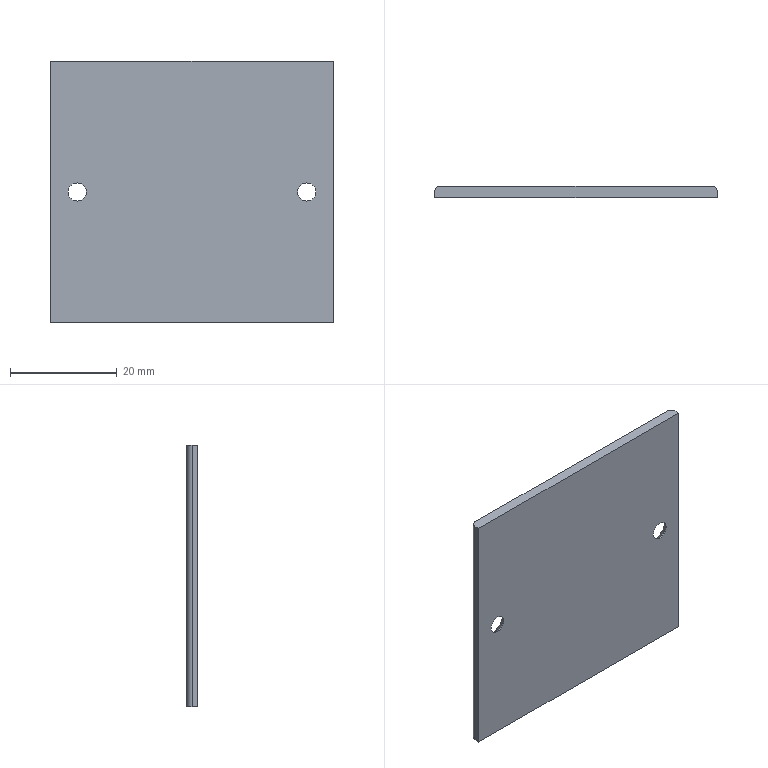Part | SolidWorks | features BaseBody 1 | 1 solid | 16 faces | box 53 x 2 x 49 mm | volume 5090 mm3 | cylinder 6 | plane 6 | cone 4 | commonest cylinder face diameters 3.4 x4 2 x2
STEP:
#1=CARTESIAN_POINT('',(21.5,-1.,-1.7));
#2=VERTEX_POINT('',#1);
#3=CARTESIAN_POINT('',(21.5,-1.,1.7));
#4=VERTEX_POINT('',#3);
#5=CARTESIAN_POINT('',(21.5,-1.,0.));
#6=DIRECTION('',(0.,1.,0.));
#7=DIRECTION('',(0.,0.,1.));
#8=AXIS2_PLACEMENT_3D('',#5,#6,#7);
#9=CIRCLE('',#8,1.7);
#10=EDGE_CURVE('',#2,#4,#9,.T.);
#11=ORIENTED_EDGE('',*,*,#10,.F.);
#12=CARTESIAN_POINT('',(21.5,-0.8,-1.7));
#13=VERTEX_POINT('',#12);
#14=CARTESIAN_POINT('',(21.5,1.,-1.7));
#15=DIRECTION('',(0.,1.,0.));
#16=VECTOR('',#15,1000.);
#17=LINE('',#14,#16);
#18=EDGE_CURVE('',#2,#13,#17,.T.);
#19=ORIENTED_EDGE('',*,*,#18,.T.);
#20=CARTESIAN_POINT('',(21.5,-0.8,1.7));
#21=VERTEX_POINT('',#20);
#22=CARTESIAN_POINT('',(21.5,-0.8,0.));
#23=DIRECTION('',(0.,-1.,0.));
#24=DIRECTION('',(0.,0.,1.));
#25=AXIS2_PLACEMENT_3D('',#22,#23,#24);
#26=CIRCLE('',#25,1.7);
#27=EDGE_CURVE('',#21,#13,#26,.T.);
#28=ORIENTED_EDGE('',*,*,#27,.F.);
#29=CARTESIAN_POINT('',(21.5,1.,1.7));
#30=DIRECTION('',(0.,1.,0.));
#31=VECTOR('',#30,1000.);
#32=LINE('',#29,#31);
#33=EDGE_CURVE('',#4,#21,#32,.T.);
#34=ORIENTED_EDGE('',*,*,#33,.F.);
#35=EDGE_LOOP('',(#11,#19,#28,#34));
#36=FACE_OUTER_BOUND('',#35,.T.);
#37=CARTESIAN_POINT('',(21.5,1.,0.));
#38=DIRECTION('',(0.,1.,0.));
#39=DIRECTION('',(0.,0.,1.));
#40=AXIS2_PLACEMENT_3D('',#37,#38,#39);
#41=CYLINDRICAL_SURFACE('',#40,1.7);
#42=ADVANCED_FACE('',(#36),#41,.F.);
#43=CARTESIAN_POINT('',(-21.5,-1.,-1.7));
#44=VERTEX_POINT('',#43);
#45=CARTESIAN_POINT('',(-21.5,-1.,1.7));
#46=VERTEX_POINT('',#45);
#47=CARTESIAN_POINT('',(-21.5,-1.,0.));
#48=DIRECTION('',(0.,1.,0.));
#49=DIRECTION('',(0.,0.,1.));
#50=AXIS2_PLACEMENT_3D('',#47,#48,#49);
#51=CIRCLE('',#50,1.7);
#52=EDGE_CURVE('',#44,#46,#51,.T.);
#53=ORIENTED_EDGE('',*,*,#52,.F.);
#54=CARTESIAN_POINT('',(-21.5,-0.8,-1.7));
#55=VERTEX_POINT('',#54);
#56=CARTESIAN_POINT('',(-21.5,1.,-1.7));
#57=DIRECTION('',(0.,1.,0.));
#58=VECTOR('',#57,1000.);
#59=LINE('',#56,#58);
#60=EDGE_CURVE('',#44,#55,#59,.T.);
#61=ORIENTED_EDGE('',*,*,#60,.T.);
#62=CARTESIAN_POINT('',(-21.5,-0.8,1.7));
#63=VERTEX_POINT('',#62);
#64=CARTESIAN_POINT('',(-21.5,-0.8,0.));
#65=DIRECTION('',(0.,-1.,0.));
#66=DIRECTION('',(0.,0.,1.));
#67=AXIS2_PLACEMENT_3D('',#64,#65,#66);
#68=CIRCLE('',#67,1.7);
#69=EDGE_CURVE('',#63,#55,#68,.T.);
#70=ORIENTED_EDGE('',*,*,#69,.F.);
#71=CARTESIAN_POINT('',(-21.5,1.,1.7));
#72=DIRECTION('',(0.,1.,0.));
#73=VECTOR('',#72,1000.);
#74=LINE('',#71,#73);
#75=EDGE_CURVE('',#46,#63,#74,.T.);
#76=ORIENTED_EDGE('',*,*,#75,.F.);
#77=EDGE_LOOP('',(#53,#61,#70,#76));
#78=FACE_OUTER_BOUND('',#77,.T.);
#79=CARTESIAN_POINT('',(-21.5,1.,0.));
#80=DIRECTION('',(0.,1.,0.));
#81=DIRECTION('',(0.,0.,1.));
#82=AXIS2_PLACEMENT_3D('',#79,#80,#81);
#83=CYLINDRICAL_SURFACE('',#82,1.7);
#84=ADVANCED_FACE('',(#78),#83,.F.);
#85=ORIENTED_EDGE('',*,*,#27,.T.);
#86=CARTESIAN_POINT('',(21.5,1.,-3.5));
#87=VERTEX_POINT('',#86);
#88=CARTESIAN_POINT('',(21.5,1.,-3.5));
#89=DIRECTION('',(0.,0.7071,-0.7071));
#90=VECTOR('',#89,1000.);
#91=LINE('',#88,#90);
#92=EDGE_CURVE('',#13,#87,#91,.T.);
#93=ORIENTED_EDGE('',*,*,#92,.T.);
#94=CARTESIAN_POINT('',(21.5,1.,3.5));
#95=VERTEX_POINT('',#94);
#96=CARTESIAN_POINT('',(21.5,1.,0.));
#97=DIRECTION('',(0.,1.,0.));
#98=DIRECTION('',(0.,0.,1.));
#99=AXIS2_PLACEMENT_3D('',#96,#97,#98);
#100=CIRCLE('',#99,3.5);
#101=EDGE_CURVE('',#87,#95,#100,.T.);
#102=ORIENTED_EDGE('',*,*,#101,.T.);
#103=CARTESIAN_POINT('',(21.5,1.,3.5));
#104=DIRECTION('',(0.,0.7071,0.7071));
#105=VECTOR('',#104,1000.);
#106=LINE('',#103,#105);
#107=EDGE_CURVE('',#21,#95,#106,.T.);
#108=ORIENTED_EDGE('',*,*,#107,.F.);
#109=EDGE_LOOP('',(#85,#93,#102,#108));
#110=FACE_OUTER_BOUND('',#109,.T.);
#111=CARTESIAN_POINT('',(21.5,1.,0.));
#112=DIRECTION('',(0.,1.,0.));
#113=DIRECTION('',(0.,0.,1.));
#114=AXIS2_PLACEMENT_3D('',#111,#112,#113);
#115=CONICAL_SURFACE('',#114,3.5,0.7854);
#116=ADVANCED_FACE('',(#110),#115,.F.);
#117=ORIENTED_EDGE('',*,*,#69,.T.);
#118=CARTESIAN_POINT('',(-21.5,1.,-3.5));
#119=VERTEX_POINT('',#118);
#120=CARTESIAN_POINT('',(-21.5,1.,-3.5));
#121=DIRECTION('',(0.,0.7071,-0.7071));
#122=VECTOR('',#121,1000.);
#123=LINE('',#120,#122);
#124=EDGE_CURVE('',#55,#119,#123,.T.);
#125=ORIENTED_EDGE('',*,*,#124,.T.);
#126=CARTESIAN_POINT('',(-21.5,1.,3.5));
#127=VERTEX_POINT('',#126);
#128=CARTESIAN_POINT('',(-21.5,1.,0.));
#129=DIRECTION('',(0.,1.,0.));
#130=DIRECTION('',(0.,0.,1.));
#131=AXIS2_PLACEMENT_3D('',#128,#129,#130);
#132=CIRCLE('',#131,3.5);
#133=EDGE_CURVE('',#119,#127,#132,.T.);
#134=ORIENTED_EDGE('',*,*,#133,.T.);
#135=CARTESIAN_POINT('',(-21.5,1.,3.5));
#136=DIRECTION('',(0.,0.7071,0.7071));
#137=VECTOR('',#136,1000.);
#138=LINE('',#135,#137);
#139=EDGE_CURVE('',#63,#127,#138,.T.);
#140=ORIENTED_EDGE('',*,*,#139,.F.);
#141=EDGE_LOOP('',(#117,#125,#134,#140));
#142=FACE_OUTER_BOUND('',#141,.T.);
#143=CARTESIAN_POINT('',(-21.5,1.,0.));
#144=DIRECTION('',(0.,1.,0.));
#145=DIRECTION('',(0.,0.,1.));
#146=AXIS2_PLACEMENT_3D('',#143,#144,#145);
#147=CONICAL_SURFACE('',#146,3.5,0.7854);
#148=ADVANCED_FACE('',(#142),#147,.F.);
#149=CARTESIAN_POINT('',(26.5,-1.,-24.5));
#150=VERTEX_POINT('',#149);
#151=CARTESIAN_POINT('',(26.5,-1.,24.5));
#152=VERTEX_POINT('',#151);
#153=CARTESIAN_POINT('',(26.5,-1.,0.));
#154=DIRECTION('',(0.,0.,1.));
#155=VECTOR('',#154,1000.);
#156=LINE('',#153,#155);
#157=EDGE_CURVE('',#150,#152,#156,.T.);
#158=ORIENTED_EDGE('',*,*,#157,.T.);
#159=CARTESIAN_POINT('',(-26.5,-1.,24.5));
#160=VERTEX_POINT('',#159);
#161=CARTESIAN_POINT('',(0.,-1.,24.5));
#162=DIRECTION('',(-1.,0.,0.));
#163=VECTOR('',#162,1000.);
#164=LINE('',#161,#163);
#165=EDGE_CURVE('',#152,#160,#164,.T.);
#166=ORIENTED_EDGE('',*,*,#165,.T.);
#167=CARTESIAN_POINT('',(-26.5,-1.,-24.5));
#168=VERTEX_POINT('',#167);
#169=CARTESIAN_POINT('',(-26.5,-1.,0.));
#170=DIRECTION('',(0.,0.,-1.));
#171=VECTOR('',#170,1000.);
#172=LINE('',#169,#171);
#173=EDGE_CURVE('',#160,#168,#172,.T.);
#174=ORIENTED_EDGE('',*,*,#173,.T.);
#175=CARTESIAN_POINT('',(0.,-1.,-24.5));
#176=DIRECTION('',(1.,0.,0.));
#177=VECTOR('',#176,1000.);
#178=LINE('',#175,#177);
#179=EDGE_CURVE('',#168,#150,#178,.T.);
#180=ORIENTED_EDGE('',*,*,#179,.T.);
#181=EDGE_LOOP('',(#158,#166,#174,#180));
#182=FACE_OUTER_BOUND('',#181,.T.);
#183=CARTESIAN_POINT('',(21.5,-1.,0.));
#184=DIRECTION('',(0.,1.,0.));
#185=DIRECTION('',(0.,0.,1.));
#186=AXIS2_PLACEMENT_3D('',#183,#184,#185);
#187=CIRCLE('',#186,1.7);
#188=EDGE_CURVE('',#4,#2,#187,.T.);
#189=ORIENTED_EDGE('',*,*,#188,.T.);
#190=ORIENTED_EDGE('',*,*,#10,.T.);
#191=EDGE_LOOP('',(#189,#190));
#192=FACE_BOUND('',#191,.T.);
#193=CARTESIAN_POINT('',(-21.5,-1.,0.));
#194=DIRECTION('',(0.,1.,0.));
#195=DIRECTION('',(0.,0.,1.));
#196=AXIS2_PLACEMENT_3D('',#193,#194,#195);
#197=CIRCLE('',#196,1.7);
#198=EDGE_CURVE('',#46,#44,#197,.T.);
#199=ORIENTED_EDGE('',*,*,#198,.T.);
#200=ORIENTED_EDGE('',*,*,#52,.T.);
#201=EDGE_LOOP('',(#199,#200));
#202=FACE_BOUND('',#201,.T.);
#203=CARTESIAN_POINT('',(0.,-1.,0.));
#204=DIRECTION('',(0.,-1.,0.));
#205=DIRECTION('',(0.,0.,-1.));
#206=AXIS2_PLACEMENT_3D('',#203,#204,#205);
#207=PLANE('',#206);
#208=ADVANCED_FACE('',(#182,#192,#202),#207,.T.);
#209=CARTESIAN_POINT('',(25.5,1.,24.5));
#210=VERTEX_POINT('',#209);
#211=CARTESIAN_POINT('',(26.5,0.,24.5));
#212=VERTEX_POINT('',#211);
#213=CARTESIAN_POINT('',(25.5,0.,24.5));
#214=DIRECTION('',(0.,0.,-1.));
#215=DIRECTION('',(-1.,0.,0.));
#216=AXIS2_PLACEMENT_3D('',#213,#214,#215);
#217=CIRCLE('',#216,1.);
#218=EDGE_CURVE('',#210,#212,#217,.T.);
#219=ORIENTED_EDGE('',*,*,#218,.F.);
#220=CARTESIAN_POINT('',(-25.5,1.,24.5));
#221=VERTEX_POINT('',#220);
#222=CARTESIAN_POINT('',(26.5,1.,24.5));
#223=DIRECTION('',(1.,0.,0.));
#224=VECTOR('',#223,1000.);
#225=LINE('',#222,#224);
#226=EDGE_CURVE('',#221,#210,#225,.T.);
#227=ORIENTED_EDGE('',*,*,#226,.F.);
#228=CARTESIAN_POINT('',(-26.5,0.,24.5));
#229=VERTEX_POINT('',#228);
#230=CARTESIAN_POINT('',(-25.5,0.,24.5));
#231=DIRECTION('',(0.,0.,-1.));
#232=DIRECTION('',(1.,0.,0.));
#233=AXIS2_PLACEMENT_3D('',#230,#231,#232);
#234=CIRCLE('',#233,1.);
#235=EDGE_CURVE('',#229,#221,#234,.T.);
#236=ORIENTED_EDGE('',*,*,#235,.F.);
#237=CARTESIAN_POINT('',(-26.5,1.,24.5));
#238=DIRECTION('',(0.,1.,0.));
#239=VECTOR('',#238,1000.);
#240=LINE('',#237,#239);
#241=EDGE_CURVE('',#160,#229,#240,.T.);
#242=ORIENTED_EDGE('',*,*,#241,.F.);
#243=ORIENTED_EDGE('',*,*,#165,.F.);
#244=CARTESIAN_POINT('',(26.5,1.,24.5));
#245=DIRECTION('',(0.,-1.,0.));
#246=VECTOR('',#245,1000.);
#247=LINE('',#244,#246);
#248=EDGE_CURVE('',#212,#152,#247,.T.);
#249=ORIENTED_EDGE('',*,*,#248,.F.);
#250=EDGE_LOOP('',(#219,#227,#236,#242,#243,#249));
#251=FACE_OUTER_BOUND('',#250,.T.);
#252=CARTESIAN_POINT('',(26.5,1.,24.5));
#253=DIRECTION('',(0.,0.,-1.));
#254=DIRECTION('',(-1.,0.,0.));
#255=AXIS2_PLACEMENT_3D('',#252,#253,#254);
#256=PLANE('',#255);
#257=ADVANCED_FACE('',(#251),#256,.F.);
#258=CARTESIAN_POINT('',(26.5,0.,-24.5));
#259=VERTEX_POINT('',#258);
#260=CARTESIAN_POINT('',(26.5,0.,-24.5));
#261=DIRECTION('',(0.,0.,-1.));
#262=VECTOR('',#261,1000.);
#263=LINE('',#260,#262);
#264=EDGE_CURVE('',#212,#259,#263,.T.);
#265=ORIENTED_EDGE('',*,*,#264,.F.);
#266=ORIENTED_EDGE('',*,*,#248,.T.);
#267=ORIENTED_EDGE('',*,*,#157,.F.);
#268=CARTESIAN_POINT('',(26.5,1.,-24.5));
#269=DIRECTION('',(0.,-1.,0.));
#270=VECTOR('',#269,1000.);
#271=LINE('',#268,#270);
#272=EDGE_CURVE('',#259,#150,#271,.T.);
#273=ORIENTED_EDGE('',*,*,#272,.F.);
#274=EDGE_LOOP('',(#265,#266,#267,#273));
#275=FACE_OUTER_BOUND('',#274,.T.);
#276=CARTESIAN_POINT('',(26.5,1.,-24.5));
#277=DIRECTION('',(-1.,0.,0.));
#278=DIRECTION('',(0.,0.,1.));
#279=AXIS2_PLACEMENT_3D('',#276,#277,#278);
#280=PLANE('',#279);
#281=ADVANCED_FACE('',(#275),#280,.F.);
#282=CARTESIAN_POINT('',(25.5,1.,-24.5));
#283=VERTEX_POINT('',#282);
#284=CARTESIAN_POINT('',(25.5,0.,-24.5));
#285=DIRECTION('',(0.,0.,1.));
#286=DIRECTION('',(-1.,0.,0.));
#287=AXIS2_PLACEMENT_3D('',#284,#285,#286);
#288=CIRCLE('',#287,1.);
#289=EDGE_CURVE('',#259,#283,#288,.T.);
#290=ORIENTED_EDGE('',*,*,#289,.F.);
#291=ORIENTED_EDGE('',*,*,#272,.T.);
#292=ORIENTED_EDGE('',*,*,#179,.F.);
#293=CARTESIAN_POINT('',(-26.5,0.,-24.5));
#294=VERTEX_POINT('',#293);
#295=CARTESIAN_POINT('',(-26.5,1.,-24.5));
#296=DIRECTION('',(0.,-1.,0.));
#297=VECTOR('',#296,1000.);
#298=LINE('',#295,#297);
#299=EDGE_CURVE('',#294,#168,#298,.T.);
#300=ORIENTED_EDGE('',*,*,#299,.F.);
#301=CARTESIAN_POINT('',(-25.5,1.,-24.5));
#302=VERTEX_POINT('',#301);
#303=CARTESIAN_POINT('',(-25.5,0.,-24.5));
#304=DIRECTION('',(0.,0.,1.));
#305=DIRECTION('',(1.,0.,0.));
#306=AXIS2_PLACEMENT_3D('',#303,#304,#305);
#307=CIRCLE('',#306,1.);
#308=EDGE_CURVE('',#302,#294,#307,.T.);
#309=ORIENTED_EDGE('',*,*,#308,.F.);
#310=CARTESIAN_POINT('',(26.5,1.,-24.5));
#311=DIRECTION('',(-1.,0.,0.));
#312=VECTOR('',#311,1000.);
#313=LINE('',#310,#312);
#314=EDGE_CURVE('',#283,#302,#313,.T.);
#315=ORIENTED_EDGE('',*,*,#314,.F.);
#316=EDGE_LOOP('',(#290,#291,#292,#300,#309,#315));
#317=FACE_OUTER_BOUND('',#316,.T.);
#318=CARTESIAN_POINT('',(26.5,1.,-24.5));
#319=DIRECTION('',(0.,0.,1.));
#320=DIRECTION('',(1.,0.,0.));
#321=AXIS2_PLACEMENT_3D('',#318,#319,#320);
#322=PLANE('',#321);
#323=ADVANCED_FACE('',(#317),#322,.F.);
#324=CARTESIAN_POINT('',(-26.5,0.,-24.5));
#325=DIRECTION('',(0.,0.,1.));
#326=VECTOR('',#325,1000.);
#327=LINE('',#324,#326);
#328=EDGE_CURVE('',#294,#229,#327,.T.);
#329=ORIENTED_EDGE('',*,*,#328,.F.);
#330=ORIENTED_EDGE('',*,*,#299,.T.);
#331=ORIENTED_EDGE('',*,*,#173,.F.);
#332=ORIENTED_EDGE('',*,*,#241,.T.);
#333=EDGE_LOOP('',(#329,#330,#331,#332));
#334=FACE_OUTER_BOUND('',#333,.T.);
#335=CARTESIAN_POINT('',(-26.5,1.,-24.5));
#336=DIRECTION('',(1.,0.,0.));
#337=DIRECTION('',(0.,0.,-1.));
#338=AXIS2_PLACEMENT_3D('',#335,#336,#337);
#339=PLANE('',#338);
#340=ADVANCED_FACE('',(#334),#339,.F.);
#341=ORIENTED_EDGE('',*,*,#18,.F.);
#342=ORIENTED_EDGE('',*,*,#188,.F.);
#343=ORIENTED_EDGE('',*,*,#33,.T.);
#344=CARTESIAN_POINT('',(21.5,-0.8,0.));
#345=DIRECTION('',(0.,-1.,0.));
#346=DIRECTION('',(0.,0.,1.));
#347=AXIS2_PLACEMENT_3D('',#344,#345,#346);
#348=CIRCLE('',#347,1.7);
#349=EDGE_CURVE('',#13,#21,#348,.T.);
#350=ORIENTED_EDGE('',*,*,#349,.F.);
#351=EDGE_LOOP('',(#341,#342,#343,#350));
#352=FACE_OUTER_BOUND('',#351,.T.);
#353=CARTESIAN_POINT('',(21.5,1.,0.));
#354=DIRECTION('',(0.,1.,0.));
#355=DIRECTION('',(0.,0.,1.));
#356=AXIS2_PLACEMENT_3D('',#353,#354,#355);
#357=CYLINDRICAL_SURFACE('',#356,1.7);
#358=ADVANCED_FACE('',(#352),#357,.F.);
#359=ORIENTED_EDGE('',*,*,#60,.F.);
#360=ORIENTED_EDGE('',*,*,#198,.F.);
#361=ORIENTED_EDGE('',*,*,#75,.T.);
#362=CARTESIAN_POINT('',(-21.5,-0.8,0.));
#363=DIRECTION('',(0.,-1.,0.));
#364=DIRECTION('',(0.,0.,1.));
#365=AXIS2_PLACEMENT_3D('',#362,#363,#364);
#366=CIRCLE('',#365,1.7);
#367=EDGE_CURVE('',#55,#63,#366,.T.);
#368=ORIENTED_EDGE('',*,*,#367,.F.);
#369=EDGE_LOOP('',(#359,#360,#361,#368));
#370=FACE_OUTER_BOUND('',#369,.T.);
#371=CARTESIAN_POINT('',(-21.5,1.,0.));
#372=DIRECTION('',(0.,1.,0.));
#373=DIRECTION('',(0.,0.,1.));
#374=AXIS2_PLACEMENT_3D('',#371,#372,#373);
#375=CYLINDRICAL_SURFACE('',#374,1.7);
#376=ADVANCED_FACE('',(#370),#375,.F.);
#377=CARTESIAN_POINT('',(25.5,1.,0.));
#378=DIRECTION('',(0.,0.,1.));
#379=VECTOR('',#378,1000.);
#380=LINE('',#377,#379);
#381=EDGE_CURVE('',#283,#210,#380,.T.);
#382=ORIENTED_EDGE('',*,*,#381,.F.);
#383=ORIENTED_EDGE('',*,*,#314,.T.);
#384=CARTESIAN_POINT('',(-25.5,1.,0.));
#385=DIRECTION('',(0.,0.,-1.));
#386=VECTOR('',#385,1000.);
#387=LINE('',#384,#386);
#388=EDGE_CURVE('',#221,#302,#387,.T.);
#389=ORIENTED_EDGE('',*,*,#388,.F.);
#390=ORIENTED_EDGE('',*,*,#226,.T.);
#391=EDGE_LOOP('',(#382,#383,#389,#390));
#392=FACE_OUTER_BOUND('',#391,.T.);
#393=CARTESIAN_POINT('',(21.5,1.,0.));
#394=DIRECTION('',(0.,1.,0.));
#395=DIRECTION('',(0.,0.,1.));
#396=AXIS2_PLACEMENT_3D('',#393,#394,#395);
#397=CIRCLE('',#396,3.5);
#398=EDGE_CURVE('',#95,#87,#397,.T.);
#399=ORIENTED_EDGE('',*,*,#398,.F.);
#400=ORIENTED_EDGE('',*,*,#101,.F.);
#401=EDGE_LOOP('',(#399,#400));
#402=FACE_BOUND('',#401,.T.);
#403=CARTESIAN_POINT('',(-21.5,1.,0.));
#404=DIRECTION('',(0.,1.,0.));
#405=DIRECTION('',(0.,0.,1.));
#406=AXIS2_PLACEMENT_3D('',#403,#404,#405);
#407=CIRCLE('',#406,3.5);
#408=EDGE_CURVE('',#127,#119,#407,.T.);
#409=ORIENTED_EDGE('',*,*,#408,.F.);
#410=ORIENTED_EDGE('',*,*,#133,.F.);
#411=EDGE_LOOP('',(#409,#410));
#412=FACE_BOUND('',#411,.T.);
#413=CARTESIAN_POINT('',(0.,1.,0.));
#414=DIRECTION('',(0.,-1.,0.));
#415=DIRECTION('',(0.,0.,-1.));
#416=AXIS2_PLACEMENT_3D('',#413,#414,#415);
#417=PLANE('',#416);
#418=ADVANCED_FACE('',(#392,#402,#412),#417,.F.);
#419=ORIENTED_EDGE('',*,*,#289,.T.);
#420=ORIENTED_EDGE('',*,*,#381,.T.);
#421=ORIENTED_EDGE('',*,*,#218,.T.);
#422=ORIENTED_EDGE('',*,*,#264,.T.);
#423=EDGE_LOOP('',(#419,#420,#421,#422));
#424=FACE_OUTER_BOUND('',#423,.T.);
#425=CARTESIAN_POINT('',(25.5,0.,0.));
#426=DIRECTION('',(0.,0.,-1.));
#427=DIRECTION('',(-1.,0.,0.));
#428=AXIS2_PLACEMENT_3D('',#425,#426,#427);
#429=CYLINDRICAL_SURFACE('',#428,1.);
#430=ADVANCED_FACE('',(#424),#429,.T.);
#431=ORIENTED_EDGE('',*,*,#235,.T.);
#432=ORIENTED_EDGE('',*,*,#388,.T.);
#433=ORIENTED_EDGE('',*,*,#308,.T.);
#434=ORIENTED_EDGE('',*,*,#328,.T.);
#435=EDGE_LOOP('',(#431,#432,#433,#434));
#436=FACE_OUTER_BOUND('',#435,.T.);
#437=CARTESIAN_POINT('',(-25.5,0.,0.));
#438=DIRECTION('',(0.,0.,1.));
#439=DIRECTION('',(1.,0.,0.));
#440=AXIS2_PLACEMENT_3D('',#437,#438,#439);
#441=CYLINDRICAL_SURFACE('',#440,1.);
#442=ADVANCED_FACE('',(#436),#441,.T.);
#443=ORIENTED_EDGE('',*,*,#92,.F.);
#444=ORIENTED_EDGE('',*,*,#349,.T.);
#445=ORIENTED_EDGE('',*,*,#107,.T.);
#446=ORIENTED_EDGE('',*,*,#398,.T.);
#447=EDGE_LOOP('',(#443,#444,#445,#446));
#448=FACE_OUTER_BOUND('',#447,.T.);
#449=CARTESIAN_POINT('',(21.5,1.,0.));
#450=DIRECTION('',(0.,1.,0.));
#451=DIRECTION('',(0.,0.,1.));
#452=AXIS2_PLACEMENT_3D('',#449,#450,#451);
#453=CONICAL_SURFACE('',#452,3.5,0.7854);
#454=ADVANCED_FACE('',(#448),#453,.F.);
#455=ORIENTED_EDGE('',*,*,#124,.F.);
#456=ORIENTED_EDGE('',*,*,#367,.T.);
#457=ORIENTED_EDGE('',*,*,#139,.T.);
#458=ORIENTED_EDGE('',*,*,#408,.T.);
#459=EDGE_LOOP('',(#455,#456,#457,#458));
#460=FACE_OUTER_BOUND('',#459,.T.);
#461=CARTESIAN_POINT('',(-21.5,1.,0.));
#462=DIRECTION('',(0.,1.,0.));
#463=DIRECTION('',(0.,0.,1.));
#464=AXIS2_PLACEMENT_3D('',#461,#462,#463);
#465=CONICAL_SURFACE('',#464,3.5,0.7854);
#466=ADVANCED_FACE('',(#460),#465,.F.);
#467=CLOSED_SHELL('',(#42,#84,#116,#148,#208,#257,#281,#323,#340,#358,#376,#418,#430,#442,#454,#466));
#468=MANIFOLD_SOLID_BREP('',#467);
#469=CARTESIAN_POINT('',(0.,0.,0.));
#470=DIRECTION('',(0.,0.,1.));
#471=DIRECTION('',(1.,0.,0.));
#472=AXIS2_PLACEMENT_3D('',#469,#470,#471);
#473=(LENGTH_UNIT()NAMED_UNIT(*)SI_UNIT(.MILLI.,.METRE.));
#474=UNCERTAINTY_MEASURE_WITH_UNIT(LENGTH_MEASURE(0.00001),#473,'','');
#475=(NAMED_UNIT(*)PLANE_ANGLE_UNIT()SI_UNIT($,.RADIAN.));
#476=(NAMED_UNIT(*)SI_UNIT($,.STERADIAN.)SOLID_ANGLE_UNIT());
#477=(GEOMETRIC_REPRESENTATION_CONTEXT(3)GLOBAL_UNCERTAINTY_ASSIGNED_CONTEXT((#474))GLOBAL_UNIT_ASSIGNED_CONTEXT((#473,#475,#476))REPRESENTATION_CONTEXT('',''));
#478=ADVANCED_BREP_SHAPE_REPRESENTATION('',(#468,#472),#477);